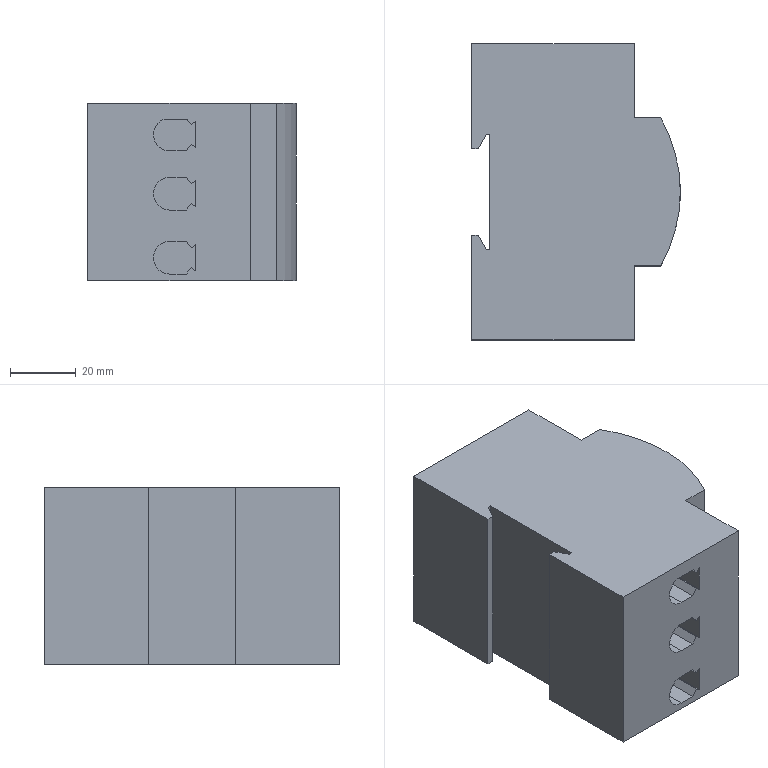Part | SolidWorks | features ICE 15, MoveFace 7, LPattern 2, Chamfer 1, CombineBodies 1, Extrusion 1, Fillet 1, MirrorPattern 1, PLine 1 | 1 solid | 151 faces | box 63.5 x 90 x 54 mm | volume 247682 mm3 | plane 133 | cylinder 18 | commonest cylinder face diameters 7 x8 10 x6 86.375 x3 90.375 x1